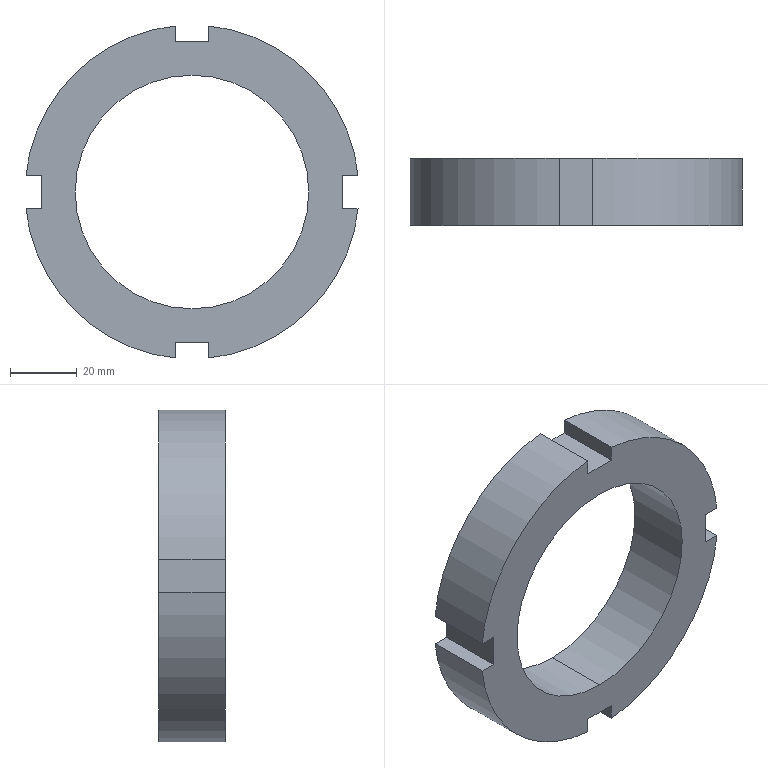Part | SolidWorks | features Extrusion 1 | 1 solid | 20 faces | box 99.499 x 20 x 99.499 mm | volume 76177 mm3 | plane 14 | cylinder 6 | commonest cylinder face diameters 100 x4 70 x2
STEP:
#1=CARTESIAN_POINT('',(0.,20.,-35.));
#2=VERTEX_POINT('',#1);
#3=CARTESIAN_POINT('',(0.,20.,35.));
#4=VERTEX_POINT('',#3);
#5=CARTESIAN_POINT('',(0.,20.,0.));
#6=DIRECTION('',(0.,1.,0.));
#7=DIRECTION('',(0.,0.,1.));
#8=AXIS2_PLACEMENT_3D('',#5,#6,#7);
#9=CIRCLE('',#8,35.);
#10=EDGE_CURVE('',#2,#4,#9,.T.);
#11=ORIENTED_EDGE('',*,*,#10,.T.);
#12=CARTESIAN_POINT('',(0.,0.,35.));
#13=VERTEX_POINT('',#12);
#14=CARTESIAN_POINT('',(0.,20.,35.));
#15=DIRECTION('',(0.,-1.,0.));
#16=VECTOR('',#15,1000.);
#17=LINE('',#14,#16);
#18=EDGE_CURVE('',#4,#13,#17,.T.);
#19=ORIENTED_EDGE('',*,*,#18,.T.);
#20=CARTESIAN_POINT('',(0.,0.,-35.));
#21=VERTEX_POINT('',#20);
#22=CARTESIAN_POINT('',(0.,0.,0.));
#23=DIRECTION('',(0.,1.,0.));
#24=DIRECTION('',(0.,0.,1.));
#25=AXIS2_PLACEMENT_3D('',#22,#23,#24);
#26=CIRCLE('',#25,35.);
#27=EDGE_CURVE('',#21,#13,#26,.T.);
#28=ORIENTED_EDGE('',*,*,#27,.F.);
#29=CARTESIAN_POINT('',(0.,20.,-35.));
#30=DIRECTION('',(0.,-1.,0.));
#31=VECTOR('',#30,1000.);
#32=LINE('',#29,#31);
#33=EDGE_CURVE('',#2,#21,#32,.T.);
#34=ORIENTED_EDGE('',*,*,#33,.F.);
#35=EDGE_LOOP('',(#11,#19,#28,#34));
#36=FACE_OUTER_BOUND('',#35,.T.);
#37=CARTESIAN_POINT('',(0.,20.,0.));
#38=DIRECTION('',(0.,-1.,0.));
#39=DIRECTION('',(0.,0.,-1.));
#40=AXIS2_PLACEMENT_3D('',#37,#38,#39);
#41=CYLINDRICAL_SURFACE('',#40,35.);
#42=ADVANCED_FACE('',(#36),#41,.F.);
#43=CARTESIAN_POINT('',(49.749,20.,-5.));
#44=VERTEX_POINT('',#43);
#45=CARTESIAN_POINT('',(5.,20.,-49.749));
#46=VERTEX_POINT('',#45);
#47=CARTESIAN_POINT('',(0.,20.,0.));
#48=DIRECTION('',(0.,1.,0.));
#49=DIRECTION('',(0.,0.,1.));
#50=AXIS2_PLACEMENT_3D('',#47,#48,#49);
#51=CIRCLE('',#50,50.);
#52=EDGE_CURVE('',#44,#46,#51,.T.);
#53=ORIENTED_EDGE('',*,*,#52,.T.);
#54=CARTESIAN_POINT('',(5.,20.,-45.));
#55=VERTEX_POINT('',#54);
#56=CARTESIAN_POINT('',(5.,20.,-45.));
#57=DIRECTION('',(0.,0.,1.));
#58=VECTOR('',#57,1000.);
#59=LINE('',#56,#58);
#60=EDGE_CURVE('',#46,#55,#59,.T.);
#61=ORIENTED_EDGE('',*,*,#60,.T.);
#62=CARTESIAN_POINT('',(-5.,20.,-45.));
#63=VERTEX_POINT('',#62);
#64=CARTESIAN_POINT('',(-5.,20.,-45.));
#65=DIRECTION('',(-1.,0.,0.));
#66=VECTOR('',#65,1000.);
#67=LINE('',#64,#66);
#68=EDGE_CURVE('',#55,#63,#67,.T.);
#69=ORIENTED_EDGE('',*,*,#68,.T.);
#70=CARTESIAN_POINT('',(-5.,20.,-49.749));
#71=VERTEX_POINT('',#70);
#72=CARTESIAN_POINT('',(-5.,20.,-49.749));
#73=DIRECTION('',(0.,0.,-1.));
#74=VECTOR('',#73,1000.);
#75=LINE('',#72,#74);
#76=EDGE_CURVE('',#63,#71,#75,.T.);
#77=ORIENTED_EDGE('',*,*,#76,.T.);
#78=CARTESIAN_POINT('',(-49.749,20.,-5.));
#79=VERTEX_POINT('',#78);
#80=CARTESIAN_POINT('',(0.,20.,0.));
#81=DIRECTION('',(0.,1.,0.));
#82=DIRECTION('',(0.,0.,1.));
#83=AXIS2_PLACEMENT_3D('',#80,#81,#82);
#84=CIRCLE('',#83,50.);
#85=EDGE_CURVE('',#71,#79,#84,.T.);
#86=ORIENTED_EDGE('',*,*,#85,.T.);
#87=CARTESIAN_POINT('',(-45.,20.,-5.));
#88=VERTEX_POINT('',#87);
#89=CARTESIAN_POINT('',(-45.,20.,-5.));
#90=DIRECTION('',(1.,0.,0.));
#91=VECTOR('',#90,1000.);
#92=LINE('',#89,#91);
#93=EDGE_CURVE('',#79,#88,#92,.T.);
#94=ORIENTED_EDGE('',*,*,#93,.T.);
#95=CARTESIAN_POINT('',(-45.,20.,5.));
#96=VERTEX_POINT('',#95);
#97=CARTESIAN_POINT('',(-45.,20.,5.));
#98=DIRECTION('',(0.,0.,1.));
#99=VECTOR('',#98,1000.);
#100=LINE('',#97,#99);
#101=EDGE_CURVE('',#88,#96,#100,.T.);
#102=ORIENTED_EDGE('',*,*,#101,.T.);
#103=CARTESIAN_POINT('',(-49.749,20.,5.));
#104=VERTEX_POINT('',#103);
#105=CARTESIAN_POINT('',(-49.749,20.,5.));
#106=DIRECTION('',(-1.,0.,0.));
#107=VECTOR('',#106,1000.);
#108=LINE('',#105,#107);
#109=EDGE_CURVE('',#96,#104,#108,.T.);
#110=ORIENTED_EDGE('',*,*,#109,.T.);
#111=CARTESIAN_POINT('',(-5.,20.,49.749));
#112=VERTEX_POINT('',#111);
#113=CARTESIAN_POINT('',(0.,20.,0.));
#114=DIRECTION('',(0.,1.,0.));
#115=DIRECTION('',(0.,0.,1.));
#116=AXIS2_PLACEMENT_3D('',#113,#114,#115);
#117=CIRCLE('',#116,50.);
#118=EDGE_CURVE('',#104,#112,#117,.T.);
#119=ORIENTED_EDGE('',*,*,#118,.T.);
#120=CARTESIAN_POINT('',(-5.,20.,45.));
#121=VERTEX_POINT('',#120);
#122=CARTESIAN_POINT('',(-5.,20.,45.));
#123=DIRECTION('',(0.,0.,-1.));
#124=VECTOR('',#123,1000.);
#125=LINE('',#122,#124);
#126=EDGE_CURVE('',#112,#121,#125,.T.);
#127=ORIENTED_EDGE('',*,*,#126,.T.);
#128=CARTESIAN_POINT('',(5.,20.,45.));
#129=VERTEX_POINT('',#128);
#130=CARTESIAN_POINT('',(5.,20.,45.));
#131=DIRECTION('',(1.,0.,0.));
#132=VECTOR('',#131,1000.);
#133=LINE('',#130,#132);
#134=EDGE_CURVE('',#121,#129,#133,.T.);
#135=ORIENTED_EDGE('',*,*,#134,.T.);
#136=CARTESIAN_POINT('',(5.,20.,49.749));
#137=VERTEX_POINT('',#136);
#138=CARTESIAN_POINT('',(5.,20.,49.749));
#139=DIRECTION('',(0.,0.,1.));
#140=VECTOR('',#139,1000.);
#141=LINE('',#138,#140);
#142=EDGE_CURVE('',#129,#137,#141,.T.);
#143=ORIENTED_EDGE('',*,*,#142,.T.);
#144=CARTESIAN_POINT('',(49.749,20.,5.));
#145=VERTEX_POINT('',#144);
#146=CARTESIAN_POINT('',(0.,20.,0.));
#147=DIRECTION('',(0.,1.,0.));
#148=DIRECTION('',(0.,0.,1.));
#149=AXIS2_PLACEMENT_3D('',#146,#147,#148);
#150=CIRCLE('',#149,50.);
#151=EDGE_CURVE('',#137,#145,#150,.T.);
#152=ORIENTED_EDGE('',*,*,#151,.T.);
#153=CARTESIAN_POINT('',(45.,20.,5.));
#154=VERTEX_POINT('',#153);
#155=CARTESIAN_POINT('',(45.,20.,5.));
#156=DIRECTION('',(-1.,0.,0.));
#157=VECTOR('',#156,1000.);
#158=LINE('',#155,#157);
#159=EDGE_CURVE('',#145,#154,#158,.T.);
#160=ORIENTED_EDGE('',*,*,#159,.T.);
#161=CARTESIAN_POINT('',(45.,20.,-5.));
#162=VERTEX_POINT('',#161);
#163=CARTESIAN_POINT('',(45.,20.,-5.));
#164=DIRECTION('',(0.,0.,-1.));
#165=VECTOR('',#164,1000.);
#166=LINE('',#163,#165);
#167=EDGE_CURVE('',#154,#162,#166,.T.);
#168=ORIENTED_EDGE('',*,*,#167,.T.);
#169=CARTESIAN_POINT('',(49.749,20.,-5.));
#170=DIRECTION('',(1.,0.,0.));
#171=VECTOR('',#170,1000.);
#172=LINE('',#169,#171);
#173=EDGE_CURVE('',#162,#44,#172,.T.);
#174=ORIENTED_EDGE('',*,*,#173,.T.);
#175=EDGE_LOOP('',(#53,#61,#69,#77,#86,#94,#102,#110,#119,#127,#135,#143,#152,#160,#168,#174));
#176=FACE_OUTER_BOUND('',#175,.T.);
#177=ORIENTED_EDGE('',*,*,#10,.F.);
#178=CARTESIAN_POINT('',(0.,20.,0.));
#179=DIRECTION('',(0.,1.,0.));
#180=DIRECTION('',(0.,0.,1.));
#181=AXIS2_PLACEMENT_3D('',#178,#179,#180);
#182=CIRCLE('',#181,35.);
#183=EDGE_CURVE('',#4,#2,#182,.T.);
#184=ORIENTED_EDGE('',*,*,#183,.F.);
#185=EDGE_LOOP('',(#177,#184));
#186=FACE_BOUND('',#185,.T.);
#187=CARTESIAN_POINT('',(0.,20.,0.));
#188=DIRECTION('',(0.,1.,0.));
#189=DIRECTION('',(0.,0.,1.));
#190=AXIS2_PLACEMENT_3D('',#187,#188,#189);
#191=PLANE('',#190);
#192=ADVANCED_FACE('',(#176,#186),#191,.T.);
#193=CARTESIAN_POINT('',(49.749,0.,-5.));
#194=VERTEX_POINT('',#193);
#195=CARTESIAN_POINT('',(5.,0.,-49.749));
#196=VERTEX_POINT('',#195);
#197=CARTESIAN_POINT('',(0.,0.,0.));
#198=DIRECTION('',(0.,1.,0.));
#199=DIRECTION('',(0.,0.,1.));
#200=AXIS2_PLACEMENT_3D('',#197,#198,#199);
#201=CIRCLE('',#200,50.);
#202=EDGE_CURVE('',#194,#196,#201,.T.);
#203=ORIENTED_EDGE('',*,*,#202,.F.);
#204=CARTESIAN_POINT('',(45.,0.,-5.));
#205=VERTEX_POINT('',#204);
#206=CARTESIAN_POINT('',(49.749,0.,-5.));
#207=DIRECTION('',(1.,0.,0.));
#208=VECTOR('',#207,1000.);
#209=LINE('',#206,#208);
#210=EDGE_CURVE('',#205,#194,#209,.T.);
#211=ORIENTED_EDGE('',*,*,#210,.F.);
#212=CARTESIAN_POINT('',(45.,0.,5.));
#213=VERTEX_POINT('',#212);
#214=CARTESIAN_POINT('',(45.,0.,-5.));
#215=DIRECTION('',(0.,0.,-1.));
#216=VECTOR('',#215,1000.);
#217=LINE('',#214,#216);
#218=EDGE_CURVE('',#213,#205,#217,.T.);
#219=ORIENTED_EDGE('',*,*,#218,.F.);
#220=CARTESIAN_POINT('',(49.749,0.,5.));
#221=VERTEX_POINT('',#220);
#222=CARTESIAN_POINT('',(45.,0.,5.));
#223=DIRECTION('',(-1.,0.,0.));
#224=VECTOR('',#223,1000.);
#225=LINE('',#222,#224);
#226=EDGE_CURVE('',#221,#213,#225,.T.);
#227=ORIENTED_EDGE('',*,*,#226,.F.);
#228=CARTESIAN_POINT('',(5.,0.,49.749));
#229=VERTEX_POINT('',#228);
#230=CARTESIAN_POINT('',(0.,0.,0.));
#231=DIRECTION('',(0.,1.,0.));
#232=DIRECTION('',(0.,0.,1.));
#233=AXIS2_PLACEMENT_3D('',#230,#231,#232);
#234=CIRCLE('',#233,50.);
#235=EDGE_CURVE('',#229,#221,#234,.T.);
#236=ORIENTED_EDGE('',*,*,#235,.F.);
#237=CARTESIAN_POINT('',(5.,0.,45.));
#238=VERTEX_POINT('',#237);
#239=CARTESIAN_POINT('',(5.,0.,49.749));
#240=DIRECTION('',(0.,0.,1.));
#241=VECTOR('',#240,1000.);
#242=LINE('',#239,#241);
#243=EDGE_CURVE('',#238,#229,#242,.T.);
#244=ORIENTED_EDGE('',*,*,#243,.F.);
#245=CARTESIAN_POINT('',(-5.,0.,45.));
#246=VERTEX_POINT('',#245);
#247=CARTESIAN_POINT('',(5.,0.,45.));
#248=DIRECTION('',(1.,0.,0.));
#249=VECTOR('',#248,1000.);
#250=LINE('',#247,#249);
#251=EDGE_CURVE('',#246,#238,#250,.T.);
#252=ORIENTED_EDGE('',*,*,#251,.F.);
#253=CARTESIAN_POINT('',(-5.,0.,49.749));
#254=VERTEX_POINT('',#253);
#255=CARTESIAN_POINT('',(-5.,0.,45.));
#256=DIRECTION('',(0.,0.,-1.));
#257=VECTOR('',#256,1000.);
#258=LINE('',#255,#257);
#259=EDGE_CURVE('',#254,#246,#258,.T.);
#260=ORIENTED_EDGE('',*,*,#259,.F.);
#261=CARTESIAN_POINT('',(-49.749,0.,5.));
#262=VERTEX_POINT('',#261);
#263=CARTESIAN_POINT('',(0.,0.,0.));
#264=DIRECTION('',(0.,1.,0.));
#265=DIRECTION('',(0.,0.,1.));
#266=AXIS2_PLACEMENT_3D('',#263,#264,#265);
#267=CIRCLE('',#266,50.);
#268=EDGE_CURVE('',#262,#254,#267,.T.);
#269=ORIENTED_EDGE('',*,*,#268,.F.);
#270=CARTESIAN_POINT('',(-45.,0.,5.));
#271=VERTEX_POINT('',#270);
#272=CARTESIAN_POINT('',(-49.749,0.,5.));
#273=DIRECTION('',(-1.,0.,0.));
#274=VECTOR('',#273,1000.);
#275=LINE('',#272,#274);
#276=EDGE_CURVE('',#271,#262,#275,.T.);
#277=ORIENTED_EDGE('',*,*,#276,.F.);
#278=CARTESIAN_POINT('',(-45.,0.,-5.));
#279=VERTEX_POINT('',#278);
#280=CARTESIAN_POINT('',(-45.,0.,5.));
#281=DIRECTION('',(0.,0.,1.));
#282=VECTOR('',#281,1000.);
#283=LINE('',#280,#282);
#284=EDGE_CURVE('',#279,#271,#283,.T.);
#285=ORIENTED_EDGE('',*,*,#284,.F.);
#286=CARTESIAN_POINT('',(-49.749,0.,-5.));
#287=VERTEX_POINT('',#286);
#288=CARTESIAN_POINT('',(-45.,0.,-5.));
#289=DIRECTION('',(1.,0.,0.));
#290=VECTOR('',#289,1000.);
#291=LINE('',#288,#290);
#292=EDGE_CURVE('',#287,#279,#291,.T.);
#293=ORIENTED_EDGE('',*,*,#292,.F.);
#294=CARTESIAN_POINT('',(-5.,0.,-49.749));
#295=VERTEX_POINT('',#294);
#296=CARTESIAN_POINT('',(0.,0.,0.));
#297=DIRECTION('',(0.,1.,0.));
#298=DIRECTION('',(0.,0.,1.));
#299=AXIS2_PLACEMENT_3D('',#296,#297,#298);
#300=CIRCLE('',#299,50.);
#301=EDGE_CURVE('',#295,#287,#300,.T.);
#302=ORIENTED_EDGE('',*,*,#301,.F.);
#303=CARTESIAN_POINT('',(-5.,0.,-45.));
#304=VERTEX_POINT('',#303);
#305=CARTESIAN_POINT('',(-5.,0.,-49.749));
#306=DIRECTION('',(0.,0.,-1.));
#307=VECTOR('',#306,1000.);
#308=LINE('',#305,#307);
#309=EDGE_CURVE('',#304,#295,#308,.T.);
#310=ORIENTED_EDGE('',*,*,#309,.F.);
#311=CARTESIAN_POINT('',(5.,0.,-45.));
#312=VERTEX_POINT('',#311);
#313=CARTESIAN_POINT('',(-5.,0.,-45.));
#314=DIRECTION('',(-1.,0.,0.));
#315=VECTOR('',#314,1000.);
#316=LINE('',#313,#315);
#317=EDGE_CURVE('',#312,#304,#316,.T.);
#318=ORIENTED_EDGE('',*,*,#317,.F.);
#319=CARTESIAN_POINT('',(5.,0.,-45.));
#320=DIRECTION('',(0.,0.,1.));
#321=VECTOR('',#320,1000.);
#322=LINE('',#319,#321);
#323=EDGE_CURVE('',#196,#312,#322,.T.);
#324=ORIENTED_EDGE('',*,*,#323,.F.);
#325=EDGE_LOOP('',(#203,#211,#219,#227,#236,#244,#252,#260,#269,#277,#285,#293,#302,#310,#318,#324));
#326=FACE_OUTER_BOUND('',#325,.T.);
#327=ORIENTED_EDGE('',*,*,#27,.T.);
#328=CARTESIAN_POINT('',(0.,0.,0.));
#329=DIRECTION('',(0.,1.,0.));
#330=DIRECTION('',(0.,0.,1.));
#331=AXIS2_PLACEMENT_3D('',#328,#329,#330);
#332=CIRCLE('',#331,35.);
#333=EDGE_CURVE('',#13,#21,#332,.T.);
#334=ORIENTED_EDGE('',*,*,#333,.T.);
#335=EDGE_LOOP('',(#327,#334));
#336=FACE_BOUND('',#335,.T.);
#337=CARTESIAN_POINT('',(0.,0.,0.));
#338=DIRECTION('',(0.,1.,0.));
#339=DIRECTION('',(0.,0.,1.));
#340=AXIS2_PLACEMENT_3D('',#337,#338,#339);
#341=PLANE('',#340);
#342=ADVANCED_FACE('',(#326,#336),#341,.F.);
#343=ORIENTED_EDGE('',*,*,#202,.T.);
#344=CARTESIAN_POINT('',(5.,20.,-49.749));
#345=DIRECTION('',(0.,-1.,0.));
#346=VECTOR('',#345,1000.);
#347=LINE('',#344,#346);
#348=EDGE_CURVE('',#46,#196,#347,.T.);
#349=ORIENTED_EDGE('',*,*,#348,.F.);
#350=ORIENTED_EDGE('',*,*,#52,.F.);
#351=CARTESIAN_POINT('',(49.749,20.,-5.));
#352=DIRECTION('',(0.,-1.,0.));
#353=VECTOR('',#352,1000.);
#354=LINE('',#351,#353);
#355=EDGE_CURVE('',#44,#194,#354,.T.);
#356=ORIENTED_EDGE('',*,*,#355,.T.);
#357=EDGE_LOOP('',(#343,#349,#350,#356));
#358=FACE_OUTER_BOUND('',#357,.T.);
#359=CARTESIAN_POINT('',(0.,20.,0.));
#360=DIRECTION('',(0.,-1.,0.));
#361=DIRECTION('',(0.,0.,-1.));
#362=AXIS2_PLACEMENT_3D('',#359,#360,#361);
#363=CYLINDRICAL_SURFACE('',#362,50.);
#364=ADVANCED_FACE('',(#358),#363,.T.);
#365=ORIENTED_EDGE('',*,*,#323,.T.);
#366=CARTESIAN_POINT('',(5.,20.,-45.));
#367=DIRECTION('',(0.,-1.,0.));
#368=VECTOR('',#367,1000.);
#369=LINE('',#366,#368);
#370=EDGE_CURVE('',#55,#312,#369,.T.);
#371=ORIENTED_EDGE('',*,*,#370,.F.);
#372=ORIENTED_EDGE('',*,*,#60,.F.);
#373=ORIENTED_EDGE('',*,*,#348,.T.);
#374=EDGE_LOOP('',(#365,#371,#372,#373));
#375=FACE_OUTER_BOUND('',#374,.T.);
#376=CARTESIAN_POINT('',(5.,20.,-45.));
#377=DIRECTION('',(1.,0.,0.));
#378=DIRECTION('',(0.,0.,-1.));
#379=AXIS2_PLACEMENT_3D('',#376,#377,#378);
#380=PLANE('',#379);
#381=ADVANCED_FACE('',(#375),#380,.F.);
#382=ORIENTED_EDGE('',*,*,#317,.T.);
#383=CARTESIAN_POINT('',(-5.,20.,-45.));
#384=DIRECTION('',(0.,-1.,0.));
#385=VECTOR('',#384,1000.);
#386=LINE('',#383,#385);
#387=EDGE_CURVE('',#63,#304,#386,.T.);
#388=ORIENTED_EDGE('',*,*,#387,.F.);
#389=ORIENTED_EDGE('',*,*,#68,.F.);
#390=ORIENTED_EDGE('',*,*,#370,.T.);
#391=EDGE_LOOP('',(#382,#388,#389,#390));
#392=FACE_OUTER_BOUND('',#391,.T.);
#393=CARTESIAN_POINT('',(-5.,20.,-45.));
#394=DIRECTION('',(0.,0.,1.));
#395=DIRECTION('',(1.,0.,0.));
#396=AXIS2_PLACEMENT_3D('',#393,#394,#395);
#397=PLANE('',#396);
#398=ADVANCED_FACE('',(#392),#397,.F.);
#399=ORIENTED_EDGE('',*,*,#309,.T.);
#400=CARTESIAN_POINT('',(-5.,20.,-49.749));
#401=DIRECTION('',(0.,-1.,0.));
#402=VECTOR('',#401,1000.);
#403=LINE('',#400,#402);
#404=EDGE_CURVE('',#71,#295,#403,.T.);
#405=ORIENTED_EDGE('',*,*,#404,.F.);
#406=ORIENTED_EDGE('',*,*,#76,.F.);
#407=ORIENTED_EDGE('',*,*,#387,.T.);
#408=EDGE_LOOP('',(#399,#405,#406,#407));
#409=FACE_OUTER_BOUND('',#408,.T.);
#410=CARTESIAN_POINT('',(-5.,20.,-49.749));
#411=DIRECTION('',(-1.,0.,0.));
#412=DIRECTION('',(0.,0.,1.));
#413=AXIS2_PLACEMENT_3D('',#410,#411,#412);
#414=PLANE('',#413);
#415=ADVANCED_FACE('',(#409),#414,.F.);
#416=ORIENTED_EDGE('',*,*,#301,.T.);
#417=CARTESIAN_POINT('',(-49.749,20.,-5.));
#418=DIRECTION('',(0.,-1.,0.));
#419=VECTOR('',#418,1000.);
#420=LINE('',#417,#419);
#421=EDGE_CURVE('',#79,#287,#420,.T.);
#422=ORIENTED_EDGE('',*,*,#421,.F.);
#423=ORIENTED_EDGE('',*,*,#85,.F.);
#424=ORIENTED_EDGE('',*,*,#404,.T.);
#425=EDGE_LOOP('',(#416,#422,#423,#424));
#426=FACE_OUTER_BOUND('',#425,.T.);
#427=CARTESIAN_POINT('',(0.,20.,0.));
#428=DIRECTION('',(0.,-1.,0.));
#429=DIRECTION('',(0.,0.,-1.));
#430=AXIS2_PLACEMENT_3D('',#427,#428,#429);
#431=CYLINDRICAL_SURFACE('',#430,50.);
#432=ADVANCED_FACE('',(#426),#431,.T.);
#433=ORIENTED_EDGE('',*,*,#292,.T.);
#434=CARTESIAN_POINT('',(-45.,20.,-5.));
#435=DIRECTION('',(0.,-1.,0.));
#436=VECTOR('',#435,1000.);
#437=LINE('',#434,#436);
#438=EDGE_CURVE('',#88,#279,#437,.T.);
#439=ORIENTED_EDGE('',*,*,#438,.F.);
#440=ORIENTED_EDGE('',*,*,#93,.F.);
#441=ORIENTED_EDGE('',*,*,#421,.T.);
#442=EDGE_LOOP('',(#433,#439,#440,#441));
#443=FACE_OUTER_BOUND('',#442,.T.);
#444=CARTESIAN_POINT('',(-45.,20.,-5.));
#445=DIRECTION('',(0.,0.,-1.));
#446=DIRECTION('',(-1.,0.,0.));
#447=AXIS2_PLACEMENT_3D('',#444,#445,#446);
#448=PLANE('',#447);
#449=ADVANCED_FACE('',(#443),#448,.F.);
#450=ORIENTED_EDGE('',*,*,#284,.T.);
#451=CARTESIAN_POINT('',(-45.,20.,5.));
#452=DIRECTION('',(0.,-1.,0.));
#453=VECTOR('',#452,1000.);
#454=LINE('',#451,#453);
#455=EDGE_CURVE('',#96,#271,#454,.T.);
#456=ORIENTED_EDGE('',*,*,#455,.F.);
#457=ORIENTED_EDGE('',*,*,#101,.F.);
#458=ORIENTED_EDGE('',*,*,#438,.T.);
#459=EDGE_LOOP('',(#450,#456,#457,#458));
#460=FACE_OUTER_BOUND('',#459,.T.);
#461=CARTESIAN_POINT('',(-45.,20.,5.));
#462=DIRECTION('',(1.,0.,0.));
#463=DIRECTION('',(0.,0.,-1.));
#464=AXIS2_PLACEMENT_3D('',#461,#462,#463);
#465=PLANE('',#464);
#466=ADVANCED_FACE('',(#460),#465,.F.);
#467=ORIENTED_EDGE('',*,*,#276,.T.);
#468=CARTESIAN_POINT('',(-49.749,20.,5.));
#469=DIRECTION('',(0.,-1.,0.));
#470=VECTOR('',#469,1000.);
#471=LINE('',#468,#470);
#472=EDGE_CURVE('',#104,#262,#471,.T.);
#473=ORIENTED_EDGE('',*,*,#472,.F.);
#474=ORIENTED_EDGE('',*,*,#109,.F.);
#475=ORIENTED_EDGE('',*,*,#455,.T.);
#476=EDGE_LOOP('',(#467,#473,#474,#475));
#477=FACE_OUTER_BOUND('',#476,.T.);
#478=CARTESIAN_POINT('',(-49.749,20.,5.));
#479=DIRECTION('',(0.,0.,1.));
#480=DIRECTION('',(1.,0.,0.));
#481=AXIS2_PLACEMENT_3D('',#478,#479,#480);
#482=PLANE('',#481);
#483=ADVANCED_FACE('',(#477),#482,.F.);
#484=ORIENTED_EDGE('',*,*,#268,.T.);
#485=CARTESIAN_POINT('',(-5.,20.,49.749));
#486=DIRECTION('',(0.,-1.,0.));
#487=VECTOR('',#486,1000.);
#488=LINE('',#485,#487);
#489=EDGE_CURVE('',#112,#254,#488,.T.);
#490=ORIENTED_EDGE('',*,*,#489,.F.);
#491=ORIENTED_EDGE('',*,*,#118,.F.);
#492=ORIENTED_EDGE('',*,*,#472,.T.);
#493=EDGE_LOOP('',(#484,#490,#491,#492));
#494=FACE_OUTER_BOUND('',#493,.T.);
#495=CARTESIAN_POINT('',(0.,20.,0.));
#496=DIRECTION('',(0.,-1.,0.));
#497=DIRECTION('',(0.,0.,-1.));
#498=AXIS2_PLACEMENT_3D('',#495,#496,#497);
#499=CYLINDRICAL_SURFACE('',#498,50.);
#500=ADVANCED_FACE('',(#494),#499,.T.);
#501=ORIENTED_EDGE('',*,*,#259,.T.);
#502=CARTESIAN_POINT('',(-5.,20.,45.));
#503=DIRECTION('',(0.,-1.,0.));
#504=VECTOR('',#503,1000.);
#505=LINE('',#502,#504);
#506=EDGE_CURVE('',#121,#246,#505,.T.);
#507=ORIENTED_EDGE('',*,*,#506,.F.);
#508=ORIENTED_EDGE('',*,*,#126,.F.);
#509=ORIENTED_EDGE('',*,*,#489,.T.);
#510=EDGE_LOOP('',(#501,#507,#508,#509));
#511=FACE_OUTER_BOUND('',#510,.T.);
#512=CARTESIAN_POINT('',(-5.,20.,45.));
#513=DIRECTION('',(-1.,0.,0.));
#514=DIRECTION('',(0.,0.,1.));
#515=AXIS2_PLACEMENT_3D('',#512,#513,#514);
#516=PLANE('',#515);
#517=ADVANCED_FACE('',(#511),#516,.F.);
#518=ORIENTED_EDGE('',*,*,#251,.T.);
#519=CARTESIAN_POINT('',(5.,20.,45.));
#520=DIRECTION('',(0.,-1.,0.));
#521=VECTOR('',#520,1000.);
#522=LINE('',#519,#521);
#523=EDGE_CURVE('',#129,#238,#522,.T.);
#524=ORIENTED_EDGE('',*,*,#523,.F.);
#525=ORIENTED_EDGE('',*,*,#134,.F.);
#526=ORIENTED_EDGE('',*,*,#506,.T.);
#527=EDGE_LOOP('',(#518,#524,#525,#526));
#528=FACE_OUTER_BOUND('',#527,.T.);
#529=CARTESIAN_POINT('',(5.,20.,45.));
#530=DIRECTION('',(0.,0.,-1.));
#531=DIRECTION('',(-1.,0.,0.));
#532=AXIS2_PLACEMENT_3D('',#529,#530,#531);
#533=PLANE('',#532);
#534=ADVANCED_FACE('',(#528),#533,.F.);
#535=ORIENTED_EDGE('',*,*,#243,.T.);
#536=CARTESIAN_POINT('',(5.,20.,49.749));
#537=DIRECTION('',(0.,-1.,0.));
#538=VECTOR('',#537,1000.);
#539=LINE('',#536,#538);
#540=EDGE_CURVE('',#137,#229,#539,.T.);
#541=ORIENTED_EDGE('',*,*,#540,.F.);
#542=ORIENTED_EDGE('',*,*,#142,.F.);
#543=ORIENTED_EDGE('',*,*,#523,.T.);
#544=EDGE_LOOP('',(#535,#541,#542,#543));
#545=FACE_OUTER_BOUND('',#544,.T.);
#546=CARTESIAN_POINT('',(5.,20.,49.749));
#547=DIRECTION('',(1.,0.,0.));
#548=DIRECTION('',(0.,0.,-1.));
#549=AXIS2_PLACEMENT_3D('',#546,#547,#548);
#550=PLANE('',#549);
#551=ADVANCED_FACE('',(#545),#550,.F.);
#552=ORIENTED_EDGE('',*,*,#235,.T.);
#553=CARTESIAN_POINT('',(49.749,20.,5.));
#554=DIRECTION('',(0.,-1.,0.));
#555=VECTOR('',#554,1000.);
#556=LINE('',#553,#555);
#557=EDGE_CURVE('',#145,#221,#556,.T.);
#558=ORIENTED_EDGE('',*,*,#557,.F.);
#559=ORIENTED_EDGE('',*,*,#151,.F.);
#560=ORIENTED_EDGE('',*,*,#540,.T.);
#561=EDGE_LOOP('',(#552,#558,#559,#560));
#562=FACE_OUTER_BOUND('',#561,.T.);
#563=CARTESIAN_POINT('',(0.,20.,0.));
#564=DIRECTION('',(0.,-1.,0.));
#565=DIRECTION('',(0.,0.,-1.));
#566=AXIS2_PLACEMENT_3D('',#563,#564,#565);
#567=CYLINDRICAL_SURFACE('',#566,50.);
#568=ADVANCED_FACE('',(#562),#567,.T.);
#569=ORIENTED_EDGE('',*,*,#226,.T.);
#570=CARTESIAN_POINT('',(45.,20.,5.));
#571=DIRECTION('',(0.,-1.,0.));
#572=VECTOR('',#571,1000.);
#573=LINE('',#570,#572);
#574=EDGE_CURVE('',#154,#213,#573,.T.);
#575=ORIENTED_EDGE('',*,*,#574,.F.);
#576=ORIENTED_EDGE('',*,*,#159,.F.);
#577=ORIENTED_EDGE('',*,*,#557,.T.);
#578=EDGE_LOOP('',(#569,#575,#576,#577));
#579=FACE_OUTER_BOUND('',#578,.T.);
#580=CARTESIAN_POINT('',(45.,20.,5.));
#581=DIRECTION('',(0.,0.,1.));
#582=DIRECTION('',(1.,0.,0.));
#583=AXIS2_PLACEMENT_3D('',#580,#581,#582);
#584=PLANE('',#583);
#585=ADVANCED_FACE('',(#579),#584,.F.);
#586=ORIENTED_EDGE('',*,*,#218,.T.);
#587=CARTESIAN_POINT('',(45.,20.,-5.));
#588=DIRECTION('',(0.,-1.,0.));
#589=VECTOR('',#588,1000.);
#590=LINE('',#587,#589);
#591=EDGE_CURVE('',#162,#205,#590,.T.);
#592=ORIENTED_EDGE('',*,*,#591,.F.);
#593=ORIENTED_EDGE('',*,*,#167,.F.);
#594=ORIENTED_EDGE('',*,*,#574,.T.);
#595=EDGE_LOOP('',(#586,#592,#593,#594));
#596=FACE_OUTER_BOUND('',#595,.T.);
#597=CARTESIAN_POINT('',(45.,20.,-5.));
#598=DIRECTION('',(-1.,0.,0.));
#599=DIRECTION('',(0.,0.,1.));
#600=AXIS2_PLACEMENT_3D('',#597,#598,#599);
#601=PLANE('',#600);
#602=ADVANCED_FACE('',(#596),#601,.F.);
#603=ORIENTED_EDGE('',*,*,#210,.T.);
#604=ORIENTED_EDGE('',*,*,#355,.F.);
#605=ORIENTED_EDGE('',*,*,#173,.F.);
#606=ORIENTED_EDGE('',*,*,#591,.T.);
#607=EDGE_LOOP('',(#603,#604,#605,#606));
#608=FACE_OUTER_BOUND('',#607,.T.);
#609=CARTESIAN_POINT('',(49.749,20.,-5.));
#610=DIRECTION('',(0.,0.,-1.));
#611=DIRECTION('',(-1.,0.,0.));
#612=AXIS2_PLACEMENT_3D('',#609,#610,#611);
#613=PLANE('',#612);
#614=ADVANCED_FACE('',(#608),#613,.F.);
#615=ORIENTED_EDGE('',*,*,#18,.F.);
#616=ORIENTED_EDGE('',*,*,#183,.T.);
#617=ORIENTED_EDGE('',*,*,#33,.T.);
#618=ORIENTED_EDGE('',*,*,#333,.F.);
#619=EDGE_LOOP('',(#615,#616,#617,#618));
#620=FACE_OUTER_BOUND('',#619,.T.);
#621=CARTESIAN_POINT('',(0.,20.,0.));
#622=DIRECTION('',(0.,-1.,0.));
#623=DIRECTION('',(0.,0.,-1.));
#624=AXIS2_PLACEMENT_3D('',#621,#622,#623);
#625=CYLINDRICAL_SURFACE('',#624,35.);
#626=ADVANCED_FACE('',(#620),#625,.F.);
#627=CLOSED_SHELL('',(#42,#192,#342,#364,#381,#398,#415,#432,#449,#466,#483,#500,#517,#534,#551,#568,#585,#602,#614,#626));
#628=MANIFOLD_SOLID_BREP('',#627);
#629=CARTESIAN_POINT('',(0.,0.,0.));
#630=DIRECTION('',(0.,0.,1.));
#631=DIRECTION('',(1.,0.,0.));
#632=AXIS2_PLACEMENT_3D('',#629,#630,#631);
#633=(LENGTH_UNIT()NAMED_UNIT(*)SI_UNIT(.MILLI.,.METRE.));
#634=UNCERTAINTY_MEASURE_WITH_UNIT(LENGTH_MEASURE(0.00001),#633,'','');
#635=(NAMED_UNIT(*)PLANE_ANGLE_UNIT()SI_UNIT($,.RADIAN.));
#636=(NAMED_UNIT(*)SI_UNIT($,.STERADIAN.)SOLID_ANGLE_UNIT());
#637=(GEOMETRIC_REPRESENTATION_CONTEXT(3)GLOBAL_UNCERTAINTY_ASSIGNED_CONTEXT((#634))GLOBAL_UNIT_ASSIGNED_CONTEXT((#633,#635,#636))REPRESENTATION_CONTEXT('',''));
#638=ADVANCED_BREP_SHAPE_REPRESENTATION('',(#628,#632),#637);